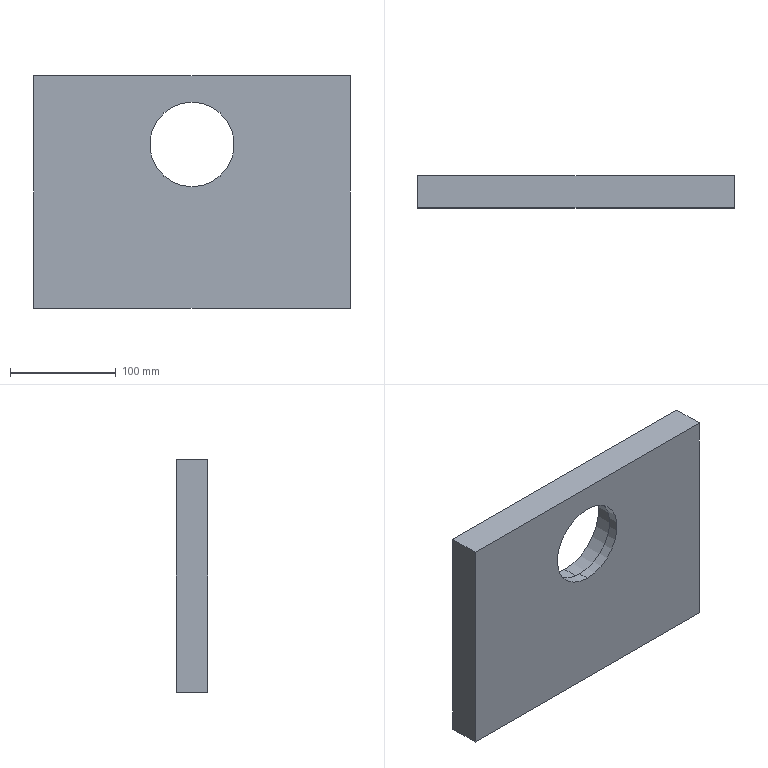Part | SolidWorks | features Cut 2, Extrusion 1 | 1 solid | 11 faces | box 300 x 30 x 220 mm | volume 1802500 mm3 | plane 7 | cylinder 4 | commonest cylinder face diameters 80 x2 90 x2
STEP:
#1=CARTESIAN_POINT('',(0.,0.,5.));
#2=VERTEX_POINT('',#1);
#3=CARTESIAN_POINT('',(0.,0.,85.));
#4=VERTEX_POINT('',#3);
#5=CARTESIAN_POINT('',(0.,0.,45.));
#6=DIRECTION('',(0.,1.,0.));
#7=DIRECTION('',(0.,0.,1.));
#8=AXIS2_PLACEMENT_3D('',#5,#6,#7);
#9=CIRCLE('',#8,40.);
#10=EDGE_CURVE('',#2,#4,#9,.T.);
#11=ORIENTED_EDGE('',*,*,#10,.F.);
#12=CARTESIAN_POINT('',(0.,10.,5.));
#13=VERTEX_POINT('',#12);
#14=CARTESIAN_POINT('',(0.,0.,5.));
#15=DIRECTION('',(0.,1.,0.));
#16=VECTOR('',#15,1000.);
#17=LINE('',#14,#16);
#18=EDGE_CURVE('',#2,#13,#17,.T.);
#19=ORIENTED_EDGE('',*,*,#18,.T.);
#20=CARTESIAN_POINT('',(0.,10.,85.));
#21=VERTEX_POINT('',#20);
#22=CARTESIAN_POINT('',(0.,10.,45.));
#23=DIRECTION('',(0.,1.,0.));
#24=DIRECTION('',(0.,0.,1.));
#25=AXIS2_PLACEMENT_3D('',#22,#23,#24);
#26=CIRCLE('',#25,40.);
#27=EDGE_CURVE('',#13,#21,#26,.T.);
#28=ORIENTED_EDGE('',*,*,#27,.T.);
#29=CARTESIAN_POINT('',(0.,0.,85.));
#30=DIRECTION('',(0.,1.,0.));
#31=VECTOR('',#30,1000.);
#32=LINE('',#29,#31);
#33=EDGE_CURVE('',#4,#21,#32,.T.);
#34=ORIENTED_EDGE('',*,*,#33,.F.);
#35=EDGE_LOOP('',(#11,#19,#28,#34));
#36=FACE_OUTER_BOUND('',#35,.T.);
#37=CARTESIAN_POINT('',(0.,0.,45.));
#38=DIRECTION('',(0.,1.,0.));
#39=DIRECTION('',(0.,0.,1.));
#40=AXIS2_PLACEMENT_3D('',#37,#38,#39);
#41=CYLINDRICAL_SURFACE('',#40,40.);
#42=ADVANCED_FACE('',(#36),#41,.F.);
#43=CARTESIAN_POINT('',(0.,10.,0.));
#44=VERTEX_POINT('',#43);
#45=CARTESIAN_POINT('',(0.,10.,90.));
#46=VERTEX_POINT('',#45);
#47=CARTESIAN_POINT('',(0.,10.,45.));
#48=DIRECTION('',(0.,1.,0.));
#49=DIRECTION('',(0.,0.,1.));
#50=AXIS2_PLACEMENT_3D('',#47,#48,#49);
#51=CIRCLE('',#50,45.);
#52=EDGE_CURVE('',#44,#46,#51,.T.);
#53=ORIENTED_EDGE('',*,*,#52,.F.);
#54=CARTESIAN_POINT('',(0.,30.,0.));
#55=VERTEX_POINT('',#54);
#56=CARTESIAN_POINT('',(0.,10.,0.));
#57=DIRECTION('',(0.,1.,0.));
#58=VECTOR('',#57,1000.);
#59=LINE('',#56,#58);
#60=EDGE_CURVE('',#44,#55,#59,.T.);
#61=ORIENTED_EDGE('',*,*,#60,.T.);
#62=CARTESIAN_POINT('',(0.,30.,90.));
#63=VERTEX_POINT('',#62);
#64=CARTESIAN_POINT('',(0.,30.,45.));
#65=DIRECTION('',(0.,1.,0.));
#66=DIRECTION('',(0.,0.,1.));
#67=AXIS2_PLACEMENT_3D('',#64,#65,#66);
#68=CIRCLE('',#67,45.);
#69=EDGE_CURVE('',#55,#63,#68,.T.);
#70=ORIENTED_EDGE('',*,*,#69,.T.);
#71=CARTESIAN_POINT('',(0.,10.,90.));
#72=DIRECTION('',(0.,1.,0.));
#73=VECTOR('',#72,1000.);
#74=LINE('',#71,#73);
#75=EDGE_CURVE('',#46,#63,#74,.T.);
#76=ORIENTED_EDGE('',*,*,#75,.F.);
#77=EDGE_LOOP('',(#53,#61,#70,#76));
#78=FACE_OUTER_BOUND('',#77,.T.);
#79=CARTESIAN_POINT('',(0.,10.,45.));
#80=DIRECTION('',(0.,1.,0.));
#81=DIRECTION('',(0.,0.,1.));
#82=AXIS2_PLACEMENT_3D('',#79,#80,#81);
#83=CYLINDRICAL_SURFACE('',#82,45.);
#84=ADVANCED_FACE('',(#78),#83,.F.);
#85=CARTESIAN_POINT('',(150.,0.,110.));
#86=VERTEX_POINT('',#85);
#87=CARTESIAN_POINT('',(150.,0.,-110.));
#88=VERTEX_POINT('',#87);
#89=CARTESIAN_POINT('',(150.,0.,110.));
#90=DIRECTION('',(0.,0.,-1.));
#91=VECTOR('',#90,1000.);
#92=LINE('',#89,#91);
#93=EDGE_CURVE('',#86,#88,#92,.T.);
#94=ORIENTED_EDGE('',*,*,#93,.T.);
#95=CARTESIAN_POINT('',(150.,30.,-110.));
#96=VERTEX_POINT('',#95);
#97=CARTESIAN_POINT('',(150.,30.,-110.));
#98=DIRECTION('',(0.,-1.,0.));
#99=VECTOR('',#98,1000.);
#100=LINE('',#97,#99);
#101=EDGE_CURVE('',#96,#88,#100,.T.);
#102=ORIENTED_EDGE('',*,*,#101,.F.);
#103=CARTESIAN_POINT('',(150.,30.,110.));
#104=VERTEX_POINT('',#103);
#105=CARTESIAN_POINT('',(150.,30.,110.));
#106=DIRECTION('',(0.,0.,-1.));
#107=VECTOR('',#106,1000.);
#108=LINE('',#105,#107);
#109=EDGE_CURVE('',#104,#96,#108,.T.);
#110=ORIENTED_EDGE('',*,*,#109,.F.);
#111=CARTESIAN_POINT('',(150.,30.,110.));
#112=DIRECTION('',(0.,-1.,0.));
#113=VECTOR('',#112,1000.);
#114=LINE('',#111,#113);
#115=EDGE_CURVE('',#104,#86,#114,.T.);
#116=ORIENTED_EDGE('',*,*,#115,.T.);
#117=EDGE_LOOP('',(#94,#102,#110,#116));
#118=FACE_OUTER_BOUND('',#117,.T.);
#119=CARTESIAN_POINT('',(150.,30.,110.));
#120=DIRECTION('',(-1.,0.,0.));
#121=DIRECTION('',(0.,0.,1.));
#122=AXIS2_PLACEMENT_3D('',#119,#120,#121);
#123=PLANE('',#122);
#124=ADVANCED_FACE('',(#118),#123,.F.);
#125=CARTESIAN_POINT('',(-150.,0.,-110.));
#126=VERTEX_POINT('',#125);
#127=CARTESIAN_POINT('',(-150.,0.,-110.));
#128=DIRECTION('',(-1.,0.,0.));
#129=VECTOR('',#128,1000.);
#130=LINE('',#127,#129);
#131=EDGE_CURVE('',#88,#126,#130,.T.);
#132=ORIENTED_EDGE('',*,*,#131,.T.);
#133=CARTESIAN_POINT('',(-150.,30.,-110.));
#134=VERTEX_POINT('',#133);
#135=CARTESIAN_POINT('',(-150.,30.,-110.));
#136=DIRECTION('',(0.,-1.,0.));
#137=VECTOR('',#136,1000.);
#138=LINE('',#135,#137);
#139=EDGE_CURVE('',#134,#126,#138,.T.);
#140=ORIENTED_EDGE('',*,*,#139,.F.);
#141=CARTESIAN_POINT('',(-150.,30.,-110.));
#142=DIRECTION('',(-1.,0.,0.));
#143=VECTOR('',#142,1000.);
#144=LINE('',#141,#143);
#145=EDGE_CURVE('',#96,#134,#144,.T.);
#146=ORIENTED_EDGE('',*,*,#145,.F.);
#147=ORIENTED_EDGE('',*,*,#101,.T.);
#148=EDGE_LOOP('',(#132,#140,#146,#147));
#149=FACE_OUTER_BOUND('',#148,.T.);
#150=CARTESIAN_POINT('',(-150.,30.,-110.));
#151=DIRECTION('',(0.,0.,1.));
#152=DIRECTION('',(1.,0.,0.));
#153=AXIS2_PLACEMENT_3D('',#150,#151,#152);
#154=PLANE('',#153);
#155=ADVANCED_FACE('',(#149),#154,.F.);
#156=CARTESIAN_POINT('',(-150.,0.,110.));
#157=VERTEX_POINT('',#156);
#158=CARTESIAN_POINT('',(-150.,0.,110.));
#159=DIRECTION('',(0.,0.,1.));
#160=VECTOR('',#159,1000.);
#161=LINE('',#158,#160);
#162=EDGE_CURVE('',#126,#157,#161,.T.);
#163=ORIENTED_EDGE('',*,*,#162,.T.);
#164=CARTESIAN_POINT('',(-150.,30.,110.));
#165=VERTEX_POINT('',#164);
#166=CARTESIAN_POINT('',(-150.,30.,110.));
#167=DIRECTION('',(0.,-1.,0.));
#168=VECTOR('',#167,1000.);
#169=LINE('',#166,#168);
#170=EDGE_CURVE('',#165,#157,#169,.T.);
#171=ORIENTED_EDGE('',*,*,#170,.F.);
#172=CARTESIAN_POINT('',(-150.,30.,110.));
#173=DIRECTION('',(0.,0.,1.));
#174=VECTOR('',#173,1000.);
#175=LINE('',#172,#174);
#176=EDGE_CURVE('',#134,#165,#175,.T.);
#177=ORIENTED_EDGE('',*,*,#176,.F.);
#178=ORIENTED_EDGE('',*,*,#139,.T.);
#179=EDGE_LOOP('',(#163,#171,#177,#178));
#180=FACE_OUTER_BOUND('',#179,.T.);
#181=CARTESIAN_POINT('',(-150.,30.,110.));
#182=DIRECTION('',(1.,0.,0.));
#183=DIRECTION('',(0.,0.,-1.));
#184=AXIS2_PLACEMENT_3D('',#181,#182,#183);
#185=PLANE('',#184);
#186=ADVANCED_FACE('',(#180),#185,.F.);
#187=CARTESIAN_POINT('',(-150.,0.,110.));
#188=DIRECTION('',(1.,0.,0.));
#189=VECTOR('',#188,1000.);
#190=LINE('',#187,#189);
#191=EDGE_CURVE('',#157,#86,#190,.T.);
#192=ORIENTED_EDGE('',*,*,#191,.T.);
#193=ORIENTED_EDGE('',*,*,#115,.F.);
#194=CARTESIAN_POINT('',(-150.,30.,110.));
#195=DIRECTION('',(1.,0.,0.));
#196=VECTOR('',#195,1000.);
#197=LINE('',#194,#196);
#198=EDGE_CURVE('',#165,#104,#197,.T.);
#199=ORIENTED_EDGE('',*,*,#198,.F.);
#200=ORIENTED_EDGE('',*,*,#170,.T.);
#201=EDGE_LOOP('',(#192,#193,#199,#200));
#202=FACE_OUTER_BOUND('',#201,.T.);
#203=CARTESIAN_POINT('',(-150.,30.,110.));
#204=DIRECTION('',(0.,0.,-1.));
#205=DIRECTION('',(-1.,0.,0.));
#206=AXIS2_PLACEMENT_3D('',#203,#204,#205);
#207=PLANE('',#206);
#208=ADVANCED_FACE('',(#202),#207,.F.);
#209=CARTESIAN_POINT('',(0.,30.,45.));
#210=DIRECTION('',(0.,1.,0.));
#211=DIRECTION('',(0.,0.,1.));
#212=AXIS2_PLACEMENT_3D('',#209,#210,#211);
#213=CIRCLE('',#212,45.);
#214=EDGE_CURVE('',#63,#55,#213,.T.);
#215=ORIENTED_EDGE('',*,*,#214,.F.);
#216=ORIENTED_EDGE('',*,*,#69,.F.);
#217=EDGE_LOOP('',(#215,#216));
#218=FACE_BOUND('',#217,.T.);
#219=ORIENTED_EDGE('',*,*,#109,.T.);
#220=ORIENTED_EDGE('',*,*,#145,.T.);
#221=ORIENTED_EDGE('',*,*,#176,.T.);
#222=ORIENTED_EDGE('',*,*,#198,.T.);
#223=EDGE_LOOP('',(#219,#220,#221,#222));
#224=FACE_OUTER_BOUND('',#223,.T.);
#225=CARTESIAN_POINT('',(0.,30.,0.));
#226=DIRECTION('',(0.,-1.,0.));
#227=DIRECTION('',(0.,0.,-1.));
#228=AXIS2_PLACEMENT_3D('',#225,#226,#227);
#229=PLANE('',#228);
#230=ADVANCED_FACE('',(#218,#224),#229,.F.);
#231=CARTESIAN_POINT('',(0.,0.,45.));
#232=DIRECTION('',(0.,1.,0.));
#233=DIRECTION('',(0.,0.,1.));
#234=AXIS2_PLACEMENT_3D('',#231,#232,#233);
#235=CIRCLE('',#234,40.);
#236=EDGE_CURVE('',#4,#2,#235,.T.);
#237=ORIENTED_EDGE('',*,*,#236,.T.);
#238=ORIENTED_EDGE('',*,*,#10,.T.);
#239=EDGE_LOOP('',(#237,#238));
#240=FACE_BOUND('',#239,.T.);
#241=ORIENTED_EDGE('',*,*,#93,.F.);
#242=ORIENTED_EDGE('',*,*,#191,.F.);
#243=ORIENTED_EDGE('',*,*,#162,.F.);
#244=ORIENTED_EDGE('',*,*,#131,.F.);
#245=EDGE_LOOP('',(#241,#242,#243,#244));
#246=FACE_OUTER_BOUND('',#245,.T.);
#247=CARTESIAN_POINT('',(0.,0.,0.));
#248=DIRECTION('',(0.,-1.,0.));
#249=DIRECTION('',(0.,0.,-1.));
#250=AXIS2_PLACEMENT_3D('',#247,#248,#249);
#251=PLANE('',#250);
#252=ADVANCED_FACE('',(#240,#246),#251,.T.);
#253=ORIENTED_EDGE('',*,*,#60,.F.);
#254=CARTESIAN_POINT('',(0.,10.,45.));
#255=DIRECTION('',(0.,1.,0.));
#256=DIRECTION('',(0.,0.,1.));
#257=AXIS2_PLACEMENT_3D('',#254,#255,#256);
#258=CIRCLE('',#257,45.);
#259=EDGE_CURVE('',#46,#44,#258,.T.);
#260=ORIENTED_EDGE('',*,*,#259,.F.);
#261=ORIENTED_EDGE('',*,*,#75,.T.);
#262=ORIENTED_EDGE('',*,*,#214,.T.);
#263=EDGE_LOOP('',(#253,#260,#261,#262));
#264=FACE_OUTER_BOUND('',#263,.T.);
#265=CARTESIAN_POINT('',(0.,10.,45.));
#266=DIRECTION('',(0.,1.,0.));
#267=DIRECTION('',(0.,0.,1.));
#268=AXIS2_PLACEMENT_3D('',#265,#266,#267);
#269=CYLINDRICAL_SURFACE('',#268,45.);
#270=ADVANCED_FACE('',(#264),#269,.F.);
#271=CARTESIAN_POINT('',(0.,10.,45.));
#272=DIRECTION('',(0.,1.,0.));
#273=DIRECTION('',(0.,0.,1.));
#274=AXIS2_PLACEMENT_3D('',#271,#272,#273);
#275=CIRCLE('',#274,40.);
#276=EDGE_CURVE('',#21,#13,#275,.T.);
#277=ORIENTED_EDGE('',*,*,#276,.F.);
#278=ORIENTED_EDGE('',*,*,#27,.F.);
#279=EDGE_LOOP('',(#277,#278));
#280=FACE_BOUND('',#279,.T.);
#281=ORIENTED_EDGE('',*,*,#259,.T.);
#282=ORIENTED_EDGE('',*,*,#52,.T.);
#283=EDGE_LOOP('',(#281,#282));
#284=FACE_OUTER_BOUND('',#283,.T.);
#285=CARTESIAN_POINT('',(0.,10.,45.));
#286=DIRECTION('',(0.,1.,0.));
#287=DIRECTION('',(0.,0.,1.));
#288=AXIS2_PLACEMENT_3D('',#285,#286,#287);
#289=PLANE('',#288);
#290=ADVANCED_FACE('',(#280,#284),#289,.T.);
#291=ORIENTED_EDGE('',*,*,#18,.F.);
#292=ORIENTED_EDGE('',*,*,#236,.F.);
#293=ORIENTED_EDGE('',*,*,#33,.T.);
#294=ORIENTED_EDGE('',*,*,#276,.T.);
#295=EDGE_LOOP('',(#291,#292,#293,#294));
#296=FACE_OUTER_BOUND('',#295,.T.);
#297=CARTESIAN_POINT('',(0.,0.,45.));
#298=DIRECTION('',(0.,1.,0.));
#299=DIRECTION('',(0.,0.,1.));
#300=AXIS2_PLACEMENT_3D('',#297,#298,#299);
#301=CYLINDRICAL_SURFACE('',#300,40.);
#302=ADVANCED_FACE('',(#296),#301,.F.);
#303=CLOSED_SHELL('',(#42,#84,#124,#155,#186,#208,#230,#252,#270,#290,#302));
#304=MANIFOLD_SOLID_BREP('',#303);
#305=CARTESIAN_POINT('',(0.,0.,0.));
#306=DIRECTION('',(0.,0.,1.));
#307=DIRECTION('',(1.,0.,0.));
#308=AXIS2_PLACEMENT_3D('',#305,#306,#307);
#309=(LENGTH_UNIT()NAMED_UNIT(*)SI_UNIT(.MILLI.,.METRE.));
#310=UNCERTAINTY_MEASURE_WITH_UNIT(LENGTH_MEASURE(0.00001),#309,'','');
#311=(NAMED_UNIT(*)PLANE_ANGLE_UNIT()SI_UNIT($,.RADIAN.));
#312=(NAMED_UNIT(*)SI_UNIT($,.STERADIAN.)SOLID_ANGLE_UNIT());
#313=(GEOMETRIC_REPRESENTATION_CONTEXT(3)GLOBAL_UNCERTAINTY_ASSIGNED_CONTEXT((#310))GLOBAL_UNIT_ASSIGNED_CONTEXT((#309,#311,#312))REPRESENTATION_CONTEXT('',''));
#314=ADVANCED_BREP_SHAPE_REPRESENTATION('',(#304,#308),#313);